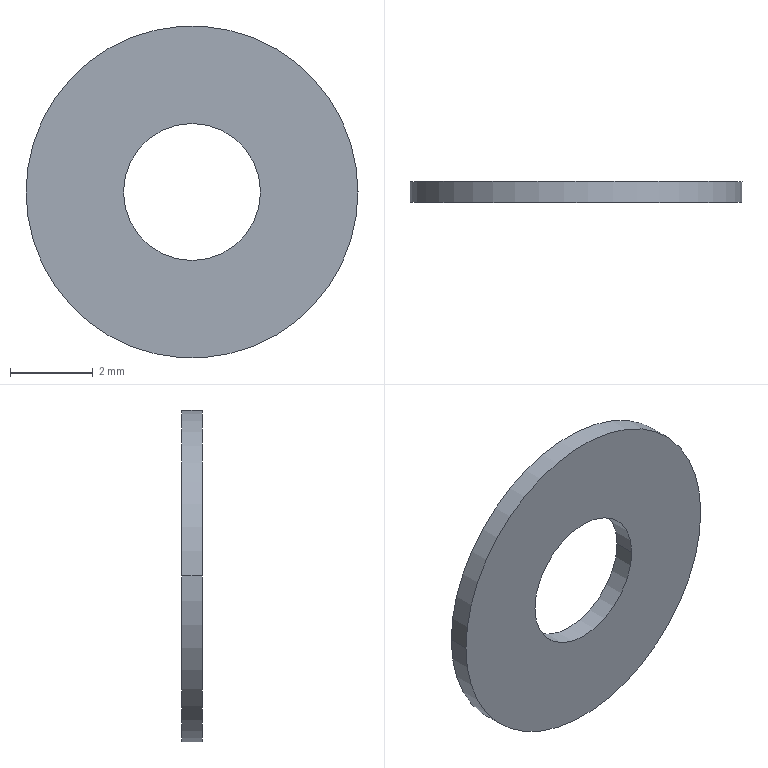Part | STEP file | ZZ21-M3-16 | 1 solid | 6 faces | box 8 x 0.5 x 8 mm | volume 20.856 mm3 | cylinder 4 | plane 2 | commonest cylinder face diameters 3.3 x2 8 x2
STEP:
#1=CARTESIAN_POINT('',(-1.65,0.,0.));
#2=VERTEX_POINT('',#1);
#3=CARTESIAN_POINT('',(1.65,0.,0.));
#4=VERTEX_POINT('',#3);
#5=CARTESIAN_POINT('',(0.,0.,0.));
#6=DIRECTION('',(0.,1.,0.));
#7=DIRECTION('',(-1.,0.,0.));
#8=AXIS2_PLACEMENT_3D('',#5,#6,#7);
#9=CIRCLE('',#8,1.65);
#10=EDGE_CURVE('',#2,#4,#9,.T.);
#11=ORIENTED_EDGE('',*,*,#10,.T.);
#12=CARTESIAN_POINT('',(1.65,-0.5,0.));
#13=VERTEX_POINT('',#12);
#14=CARTESIAN_POINT('',(1.65,0.,0.));
#15=DIRECTION('',(0.,-1.,0.));
#16=VECTOR('',#15,1000.);
#17=LINE('',#14,#16);
#18=EDGE_CURVE('',#4,#13,#17,.T.);
#19=ORIENTED_EDGE('',*,*,#18,.T.);
#20=CARTESIAN_POINT('',(-1.65,-0.5,0.));
#21=VERTEX_POINT('',#20);
#22=CARTESIAN_POINT('',(0.,-0.5,0.));
#23=DIRECTION('',(0.,-1.,0.));
#24=DIRECTION('',(1.,0.,0.));
#25=AXIS2_PLACEMENT_3D('',#22,#23,#24);
#26=CIRCLE('',#25,1.65);
#27=EDGE_CURVE('',#13,#21,#26,.T.);
#28=ORIENTED_EDGE('',*,*,#27,.T.);
#29=CARTESIAN_POINT('',(-1.65,0.,0.));
#30=DIRECTION('',(0.,-1.,0.));
#31=VECTOR('',#30,1000.);
#32=LINE('',#29,#31);
#33=EDGE_CURVE('',#2,#21,#32,.T.);
#34=ORIENTED_EDGE('',*,*,#33,.F.);
#35=EDGE_LOOP('',(#11,#19,#28,#34));
#36=FACE_OUTER_BOUND('',#35,.T.);
#37=CARTESIAN_POINT('',(0.,0.,0.));
#38=DIRECTION('',(0.,-1.,0.));
#39=DIRECTION('',(-1.,0.,0.));
#40=AXIS2_PLACEMENT_3D('',#37,#38,#39);
#41=CYLINDRICAL_SURFACE('',#40,1.65);
#42=ADVANCED_FACE('',(#36),#41,.F.);
#43=CARTESIAN_POINT('',(4.,0.,0.));
#44=VERTEX_POINT('',#43);
#45=CARTESIAN_POINT('',(-4.,0.,0.));
#46=VERTEX_POINT('',#45);
#47=CARTESIAN_POINT('',(0.,0.,0.));
#48=DIRECTION('',(0.,1.,0.));
#49=DIRECTION('',(-1.,0.,0.));
#50=AXIS2_PLACEMENT_3D('',#47,#48,#49);
#51=CIRCLE('',#50,4.);
#52=EDGE_CURVE('',#44,#46,#51,.T.);
#53=ORIENTED_EDGE('',*,*,#52,.F.);
#54=CARTESIAN_POINT('',(4.,-0.5,0.));
#55=VERTEX_POINT('',#54);
#56=CARTESIAN_POINT('',(4.,0.,0.));
#57=DIRECTION('',(0.,-1.,0.));
#58=VECTOR('',#57,1000.);
#59=LINE('',#56,#58);
#60=EDGE_CURVE('',#44,#55,#59,.T.);
#61=ORIENTED_EDGE('',*,*,#60,.T.);
#62=CARTESIAN_POINT('',(-4.,-0.5,0.));
#63=VERTEX_POINT('',#62);
#64=CARTESIAN_POINT('',(0.,-0.5,0.));
#65=DIRECTION('',(0.,-1.,0.));
#66=DIRECTION('',(1.,0.,0.));
#67=AXIS2_PLACEMENT_3D('',#64,#65,#66);
#68=CIRCLE('',#67,4.);
#69=EDGE_CURVE('',#63,#55,#68,.T.);
#70=ORIENTED_EDGE('',*,*,#69,.F.);
#71=CARTESIAN_POINT('',(-4.,0.,0.));
#72=DIRECTION('',(0.,-1.,0.));
#73=VECTOR('',#72,1000.);
#74=LINE('',#71,#73);
#75=EDGE_CURVE('',#46,#63,#74,.T.);
#76=ORIENTED_EDGE('',*,*,#75,.F.);
#77=EDGE_LOOP('',(#53,#61,#70,#76));
#78=FACE_OUTER_BOUND('',#77,.T.);
#79=CARTESIAN_POINT('',(0.,0.,0.));
#80=DIRECTION('',(0.,-1.,0.));
#81=DIRECTION('',(-1.,0.,0.));
#82=AXIS2_PLACEMENT_3D('',#79,#80,#81);
#83=CYLINDRICAL_SURFACE('',#82,4.);
#84=ADVANCED_FACE('',(#78),#83,.T.);
#85=CARTESIAN_POINT('',(0.,-0.5,0.));
#86=DIRECTION('',(0.,-1.,0.));
#87=DIRECTION('',(1.,0.,0.));
#88=AXIS2_PLACEMENT_3D('',#85,#86,#87);
#89=CIRCLE('',#88,1.65);
#90=EDGE_CURVE('',#21,#13,#89,.T.);
#91=ORIENTED_EDGE('',*,*,#90,.F.);
#92=ORIENTED_EDGE('',*,*,#27,.F.);
#93=EDGE_LOOP('',(#91,#92));
#94=FACE_BOUND('',#93,.T.);
#95=ORIENTED_EDGE('',*,*,#69,.T.);
#96=CARTESIAN_POINT('',(0.,-0.5,0.));
#97=DIRECTION('',(0.,-1.,0.));
#98=DIRECTION('',(1.,0.,0.));
#99=AXIS2_PLACEMENT_3D('',#96,#97,#98);
#100=CIRCLE('',#99,4.);
#101=EDGE_CURVE('',#55,#63,#100,.T.);
#102=ORIENTED_EDGE('',*,*,#101,.T.);
#103=EDGE_LOOP('',(#95,#102));
#104=FACE_OUTER_BOUND('',#103,.T.);
#105=CARTESIAN_POINT('',(0.,-0.5,0.));
#106=DIRECTION('',(0.,-1.,0.));
#107=DIRECTION('',(-1.,0.,0.));
#108=AXIS2_PLACEMENT_3D('',#105,#106,#107);
#109=PLANE('',#108);
#110=ADVANCED_FACE('',(#94,#104),#109,.T.);
#111=ORIENTED_EDGE('',*,*,#10,.F.);
#112=CARTESIAN_POINT('',(0.,0.,0.));
#113=DIRECTION('',(0.,1.,0.));
#114=DIRECTION('',(-1.,0.,0.));
#115=AXIS2_PLACEMENT_3D('',#112,#113,#114);
#116=CIRCLE('',#115,1.65);
#117=EDGE_CURVE('',#4,#2,#116,.T.);
#118=ORIENTED_EDGE('',*,*,#117,.F.);
#119=EDGE_LOOP('',(#111,#118));
#120=FACE_BOUND('',#119,.T.);
#121=CARTESIAN_POINT('',(0.,0.,0.));
#122=DIRECTION('',(0.,1.,0.));
#123=DIRECTION('',(-1.,0.,0.));
#124=AXIS2_PLACEMENT_3D('',#121,#122,#123);
#125=CIRCLE('',#124,4.);
#126=EDGE_CURVE('',#46,#44,#125,.T.);
#127=ORIENTED_EDGE('',*,*,#126,.T.);
#128=ORIENTED_EDGE('',*,*,#52,.T.);
#129=EDGE_LOOP('',(#127,#128));
#130=FACE_OUTER_BOUND('',#129,.T.);
#131=CARTESIAN_POINT('',(0.,0.,0.));
#132=DIRECTION('',(0.,1.,0.));
#133=DIRECTION('',(1.,0.,0.));
#134=AXIS2_PLACEMENT_3D('',#131,#132,#133);
#135=PLANE('',#134);
#136=ADVANCED_FACE('',(#120,#130),#135,.T.);
#137=ORIENTED_EDGE('',*,*,#60,.F.);
#138=ORIENTED_EDGE('',*,*,#126,.F.);
#139=ORIENTED_EDGE('',*,*,#75,.T.);
#140=ORIENTED_EDGE('',*,*,#101,.F.);
#141=EDGE_LOOP('',(#137,#138,#139,#140));
#142=FACE_OUTER_BOUND('',#141,.T.);
#143=CARTESIAN_POINT('',(0.,0.,0.));
#144=DIRECTION('',(0.,-1.,0.));
#145=DIRECTION('',(-1.,0.,0.));
#146=AXIS2_PLACEMENT_3D('',#143,#144,#145);
#147=CYLINDRICAL_SURFACE('',#146,4.);
#148=ADVANCED_FACE('',(#142),#147,.T.);
#149=ORIENTED_EDGE('',*,*,#18,.F.);
#150=ORIENTED_EDGE('',*,*,#117,.T.);
#151=ORIENTED_EDGE('',*,*,#33,.T.);
#152=ORIENTED_EDGE('',*,*,#90,.T.);
#153=EDGE_LOOP('',(#149,#150,#151,#152));
#154=FACE_OUTER_BOUND('',#153,.T.);
#155=CARTESIAN_POINT('',(0.,0.,0.));
#156=DIRECTION('',(0.,-1.,0.));
#157=DIRECTION('',(-1.,0.,0.));
#158=AXIS2_PLACEMENT_3D('',#155,#156,#157);
#159=CYLINDRICAL_SURFACE('',#158,1.65);
#160=ADVANCED_FACE('',(#154),#159,.F.);
#161=CLOSED_SHELL('',(#42,#84,#110,#136,#148,#160));
#162=MANIFOLD_SOLID_BREP('',#161);
#163=CARTESIAN_POINT('',(0.,0.,0.));
#164=DIRECTION('',(0.,0.,1.));
#165=DIRECTION('',(1.,0.,0.));
#166=AXIS2_PLACEMENT_3D('',#163,#164,#165);
#167=(LENGTH_UNIT()NAMED_UNIT(*)SI_UNIT(.MILLI.,.METRE.));
#168=UNCERTAINTY_MEASURE_WITH_UNIT(LENGTH_MEASURE(0.00001),#167,'','');
#169=(NAMED_UNIT(*)PLANE_ANGLE_UNIT()SI_UNIT($,.RADIAN.));
#170=(NAMED_UNIT(*)SI_UNIT($,.STERADIAN.)SOLID_ANGLE_UNIT());
#171=(GEOMETRIC_REPRESENTATION_CONTEXT(3)GLOBAL_UNCERTAINTY_ASSIGNED_CONTEXT((#168))GLOBAL_UNIT_ASSIGNED_CONTEXT((#167,#169,#170))REPRESENTATION_CONTEXT('',''));
#172=ADVANCED_BREP_SHAPE_REPRESENTATION('',(#162,#166),#171);